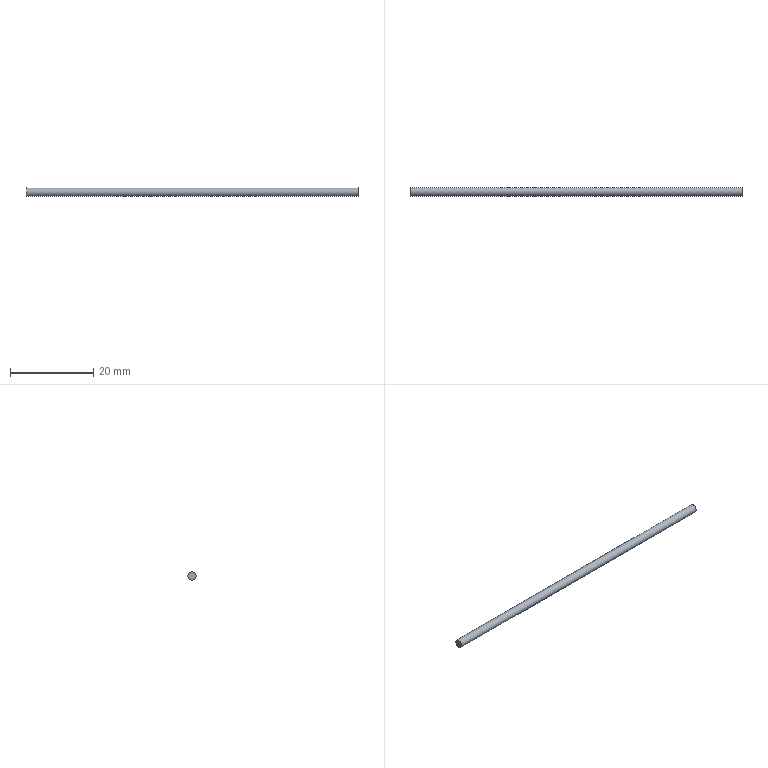Part | STEP file | 1-33.2 | 1 solid | 3 faces | box 80 x 2 x 2 mm | volume 251.327 mm3 | plane 2 | cylinder 1 | commonest cylinder face diameters 2 x1
STEP:
#1=CARTESIAN_POINT('',(0.,0.,0.));
#2=DIRECTION('',(0.,0.,1.));
#3=DIRECTION('',(1.,0.,0.));
#4=AXIS2_PLACEMENT_3D('',#1,#2,#3);
#5=CARTESIAN_POINT('',(-40.,1.,0.));
#6=VERTEX_POINT('',#5);
#7=CARTESIAN_POINT('',(-40.,0.,0.));
#8=DIRECTION('',(1.,0.,0.));
#9=DIRECTION('',(0.,1.,0.));
#10=AXIS2_PLACEMENT_3D('',#7,#8,#9);
#11=CIRCLE('',#10,1.);
#12=CARTESIAN_POINT('',(-40.,-0.2679,0.));
#13=DIRECTION('',(1.,0.,0.));
#14=DIRECTION('',(0.,1.,0.));
#15=AXIS2_PLACEMENT_3D('',#12,#13,#14);
#16=PLANE('',#15);
#17=CARTESIAN_POINT('',(0.2679,0.));
#18=DIRECTION('',(1.,0.));
#19=AXIS2_PLACEMENT_2D('',#17,#18);
#20=CIRCLE('',#19,1.);
#21=(GEOMETRIC_REPRESENTATION_CONTEXT(2)PARAMETRIC_REPRESENTATION_CONTEXT()REPRESENTATION_CONTEXT('',''));
#22=DEFINITIONAL_REPRESENTATION('',(#20),#21);
#23=PCURVE('',#16,#22);
#24=CARTESIAN_POINT('',(-40.,0.,0.));
#25=DIRECTION('',(1.,0.,0.));
#26=DIRECTION('',(0.,1.,0.));
#27=AXIS2_PLACEMENT_3D('',#24,#25,#26);
#28=CYLINDRICAL_SURFACE('',#27,1.);
#29=CARTESIAN_POINT('',(0.,0.));
#30=DIRECTION('',(1.,0.));
#31=VECTOR('',#30,1.);
#32=LINE('',#29,#31);
#33=(GEOMETRIC_REPRESENTATION_CONTEXT(2)PARAMETRIC_REPRESENTATION_CONTEXT()REPRESENTATION_CONTEXT('',''));
#34=DEFINITIONAL_REPRESENTATION('',(#32),#33);
#35=PCURVE('',#28,#34);
#36=SURFACE_CURVE('',#11,(#23,#35),.PCURVE_S1.);
#37=EDGE_CURVE('',#6,#6,#36,.T.);
#38=ORIENTED_EDGE('',*,*,#37,.T.);
#39=EDGE_LOOP('',(#38));
#40=FACE_BOUND('',#39,.F.);
#41=ADVANCED_FACE('',(#40),#16,.F.);
#42=CARTESIAN_POINT('',(40.,1.,0.));
#43=VERTEX_POINT('',#42);
#44=CARTESIAN_POINT('',(40.,0.,0.));
#45=DIRECTION('',(1.,0.,0.));
#46=DIRECTION('',(0.,1.,0.));
#47=AXIS2_PLACEMENT_3D('',#44,#45,#46);
#48=CIRCLE('',#47,1.);
#49=CARTESIAN_POINT('',(40.,-0.2679,0.));
#50=DIRECTION('',(1.,0.,0.));
#51=DIRECTION('',(0.,1.,0.));
#52=AXIS2_PLACEMENT_3D('',#49,#50,#51);
#53=PLANE('',#52);
#54=CARTESIAN_POINT('',(0.2679,0.));
#55=DIRECTION('',(1.,0.));
#56=AXIS2_PLACEMENT_2D('',#54,#55);
#57=CIRCLE('',#56,1.);
#58=(GEOMETRIC_REPRESENTATION_CONTEXT(2)PARAMETRIC_REPRESENTATION_CONTEXT()REPRESENTATION_CONTEXT('',''));
#59=DEFINITIONAL_REPRESENTATION('',(#57),#58);
#60=PCURVE('',#53,#59);
#61=CARTESIAN_POINT('',(0.,80.));
#62=DIRECTION('',(1.,0.));
#63=VECTOR('',#62,1.);
#64=LINE('',#61,#63);
#65=(GEOMETRIC_REPRESENTATION_CONTEXT(2)PARAMETRIC_REPRESENTATION_CONTEXT()REPRESENTATION_CONTEXT('',''));
#66=DEFINITIONAL_REPRESENTATION('',(#64),#65);
#67=PCURVE('',#28,#66);
#68=SURFACE_CURVE('',#48,(#60,#67),.PCURVE_S1.);
#69=EDGE_CURVE('',#43,#43,#68,.T.);
#70=ORIENTED_EDGE('',*,*,#69,.T.);
#71=EDGE_LOOP('',(#70));
#72=FACE_BOUND('',#71,.T.);
#73=ADVANCED_FACE('',(#72),#53,.T.);
#74=ORIENTED_EDGE('',*,*,#37,.T.);
#75=CARTESIAN_POINT('',(-40.,1.,0.));
#76=DIRECTION('',(1.,0.,0.));
#77=VECTOR('',#76,1.);
#78=LINE('',#75,#77);
#79=CARTESIAN_POINT('',(6.283,0.));
#80=DIRECTION('',(0.,1.));
#81=VECTOR('',#80,1.);
#82=LINE('',#79,#81);
#83=(GEOMETRIC_REPRESENTATION_CONTEXT(2)PARAMETRIC_REPRESENTATION_CONTEXT()REPRESENTATION_CONTEXT('',''));
#84=DEFINITIONAL_REPRESENTATION('',(#82),#83);
#85=PCURVE('',#28,#84);
#86=CARTESIAN_POINT('',(0.,0.));
#87=DIRECTION('',(0.,1.));
#88=VECTOR('',#87,1.);
#89=LINE('',#86,#88);
#90=(GEOMETRIC_REPRESENTATION_CONTEXT(2)PARAMETRIC_REPRESENTATION_CONTEXT()REPRESENTATION_CONTEXT('',''));
#91=DEFINITIONAL_REPRESENTATION('',(#89),#90);
#92=PCURVE('',#28,#91);
#93=SEAM_CURVE('',#78,(#85,#92),.PCURVE_S1.);
#94=EDGE_CURVE('',#6,#43,#93,.T.);
#95=ORIENTED_EDGE('',*,*,#94,.T.);
#96=ORIENTED_EDGE('',*,*,#69,.F.);
#97=ORIENTED_EDGE('',*,*,#94,.F.);
#98=EDGE_LOOP('',(#74,#95,#96,#97));
#99=FACE_BOUND('',#98,.T.);
#100=ADVANCED_FACE('',(#99),#28,.T.);
#101=CLOSED_SHELL('',(#41,#73,#100));
#102=MANIFOLD_SOLID_BREP('',#101);
#103=(LENGTH_UNIT()NAMED_UNIT(*)SI_UNIT(.MILLI.,.METRE.));
#104=UNCERTAINTY_MEASURE_WITH_UNIT(LENGTH_MEASURE(0.0000001),#103,'','');
#105=(NAMED_UNIT(*)PLANE_ANGLE_UNIT()SI_UNIT($,.RADIAN.));
#106=(NAMED_UNIT(*)SI_UNIT($,.STERADIAN.)SOLID_ANGLE_UNIT());
#107=(GEOMETRIC_REPRESENTATION_CONTEXT(3)GLOBAL_UNCERTAINTY_ASSIGNED_CONTEXT((#104))GLOBAL_UNIT_ASSIGNED_CONTEXT((#103,#105,#106))REPRESENTATION_CONTEXT('',''));
#108=ADVANCED_BREP_SHAPE_REPRESENTATION('',(#4,#102),#107);